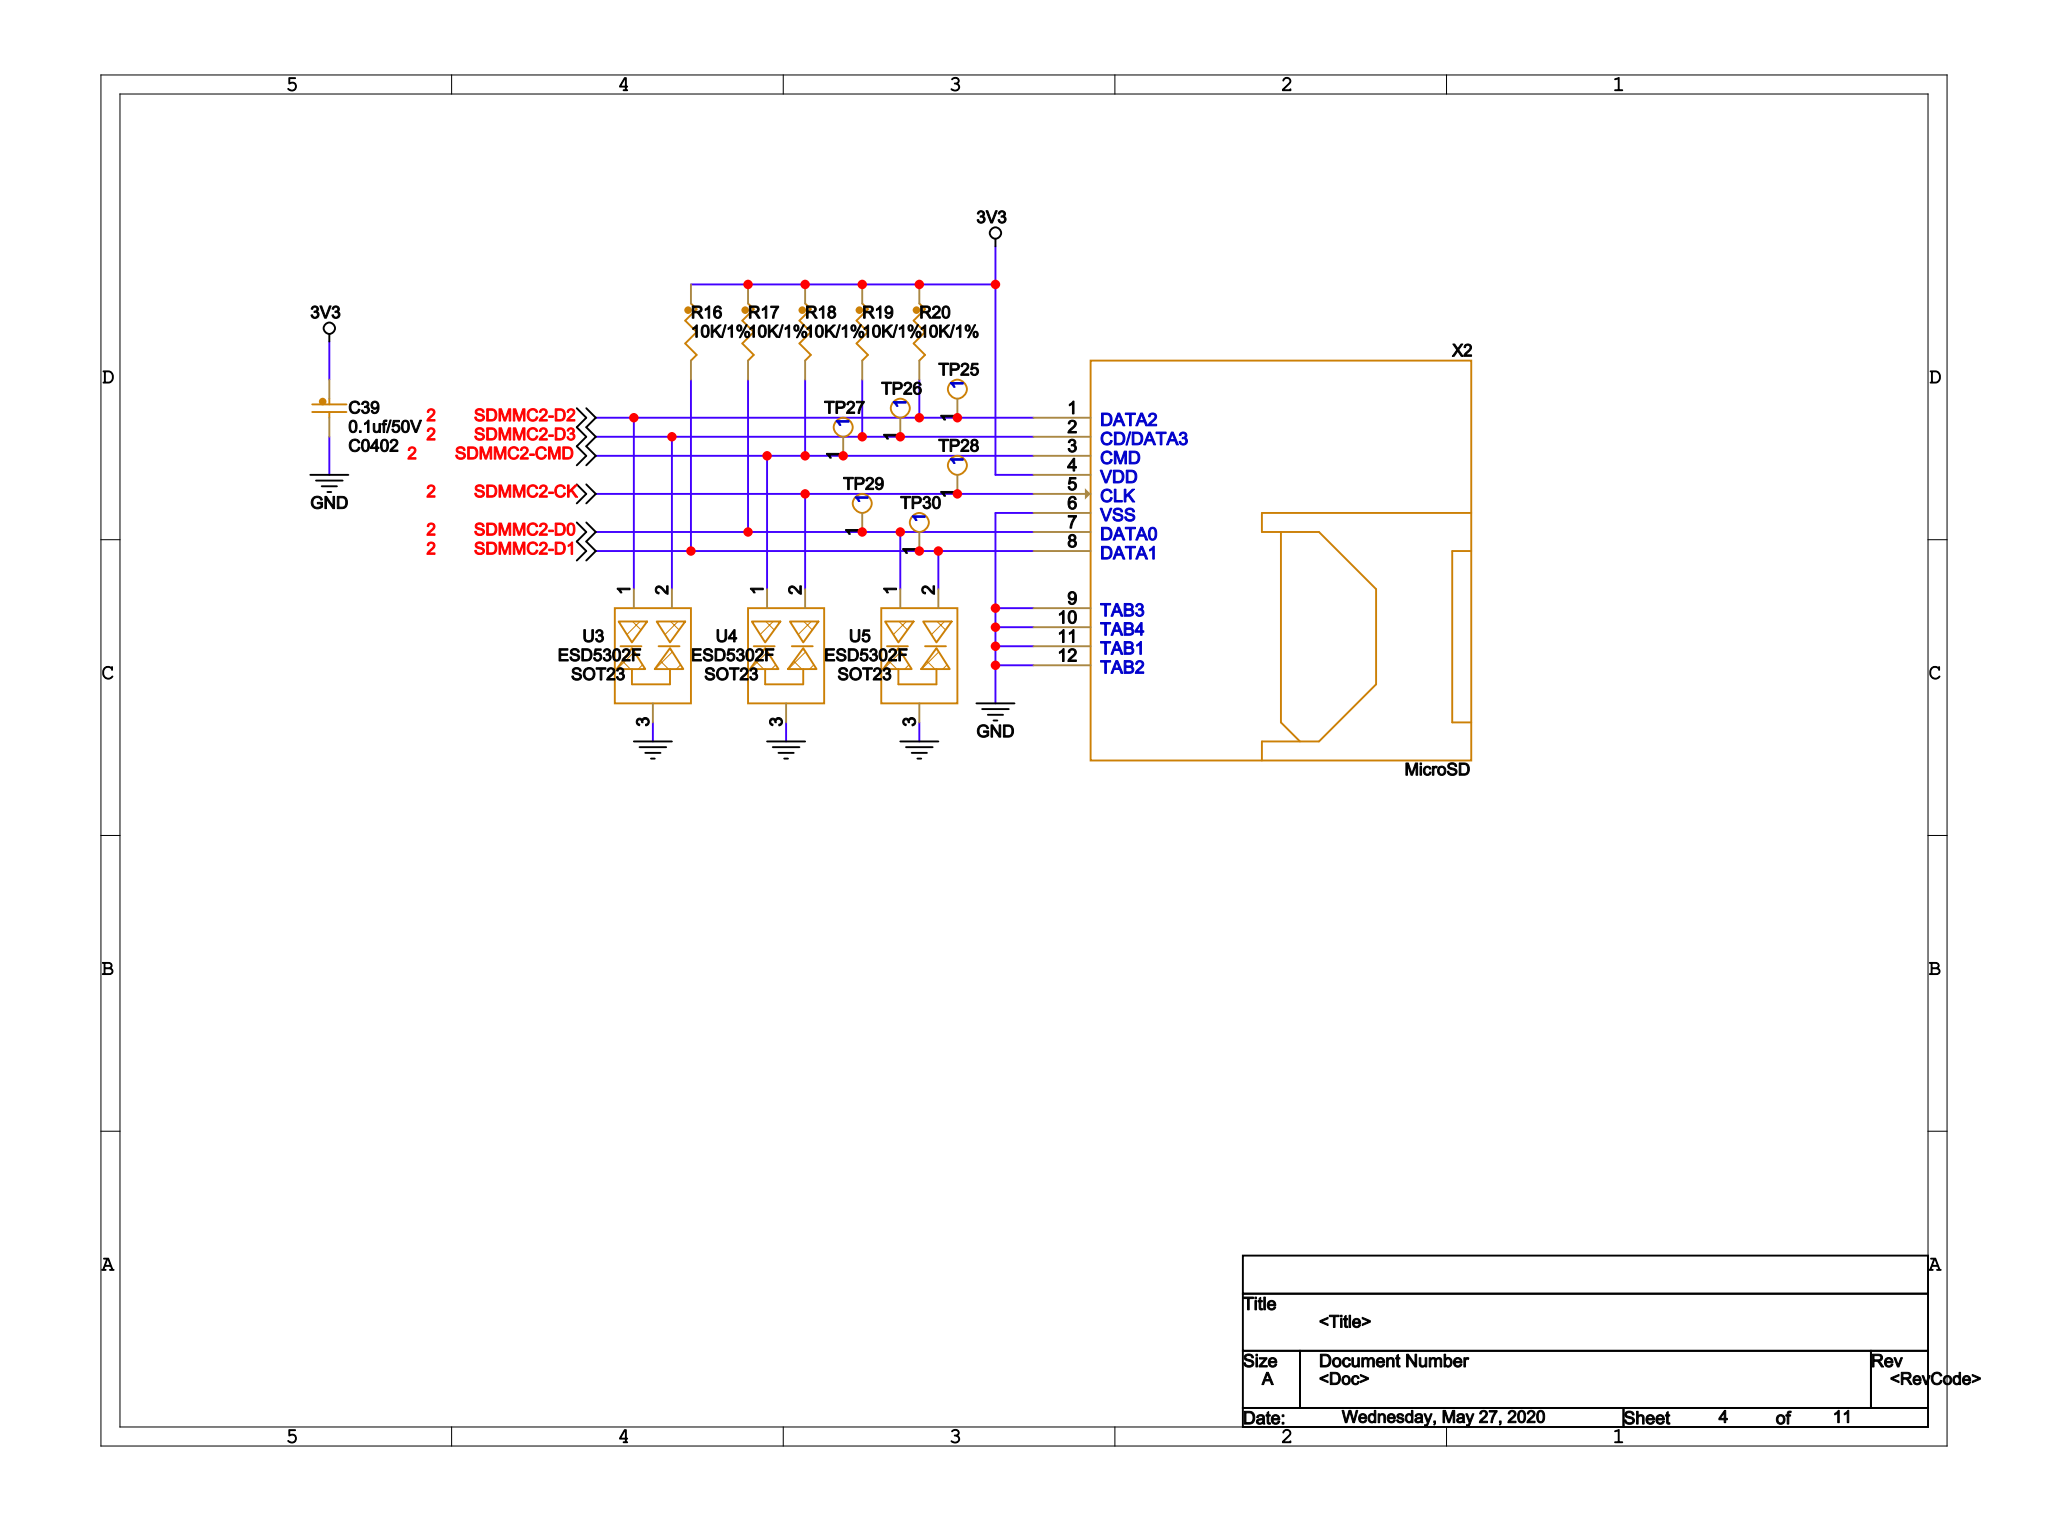Circuit board | Cadence Allegro | 521 parts | 239 nets | one sheet of the schematic
Parts on this sheet (reference | value | footprint):
C39 | 0.1uf/50V | C0402
R16 | 10K/1% | 0402
R17 | 10K/1% | 0402
R18 | 10K/1% | 0402
R19 | 10K/1% | 0402
R20 | 10K/1% | 0402
TP25 | TESTPOINT | TESTPOINT-33MIL
TP26 | TESTPOINT | TESTPOINT-33MIL
TP27 | TESTPOINT | TESTPOINT-33MIL
TP28 | TESTPOINT | TESTPOINT-33MIL
TP29 | TESTPOINT | TESTPOINT-33MIL
TP30 | TESTPOINT | TESTPOINT-33MIL
U3 | ESD5302F | SOT23
U4 | ESD5302F | SOT23
U5 | ESD5302F | SOT23
X2 | MicroSD | TFCARD-TF-02A
Nets of these parts (net: part-pin ...):
GND: C39-2 U3-3 U4-3 U5-3 X2-6 X2-9 X2-10 X2-11 X2-12
3V3: C39-1 R16-1 R17-1 R18-1 R19-1 R20-1 X2-4
SDMMC2-D2: R20-2 TP25-1 U3-1 X2-1
SDMMC2-D3: R19-2 TP26-1 U3-2 X2-2
SDMMC2-CMD: R18-2 TP27-1 U4-1 X2-3
SDMMC2-CK: TP28-1 U4-2 X2-5
SDMMC2-D0: R17-2 TP29-1 U5-1 X2-7
SDMMC2-D1: R16-2 TP30-1 U5-2 X2-8